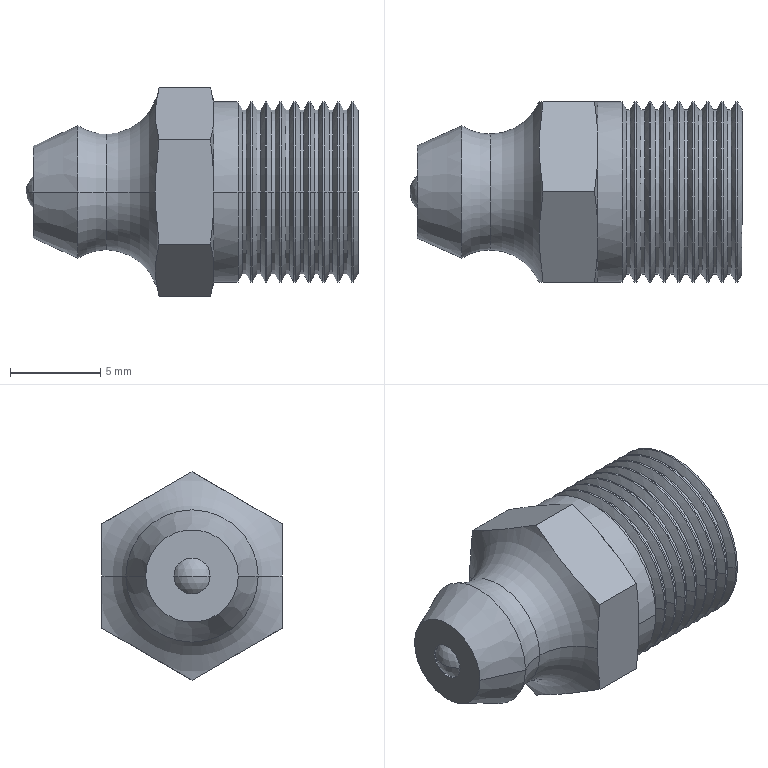Part | SolidWorks | features Cut 1, Revolution 1 | 15 solids | 167 faces | box 18.4 x 10 x 11.547 mm | volume 670.595 mm3 | torus 60 | cone 48 | cylinder 42 | plane 15 | sphere 2 | commonest cylinder face diameters 10 x18 9.134 x16 6.63 x4 2.007 x2 4.63 x2